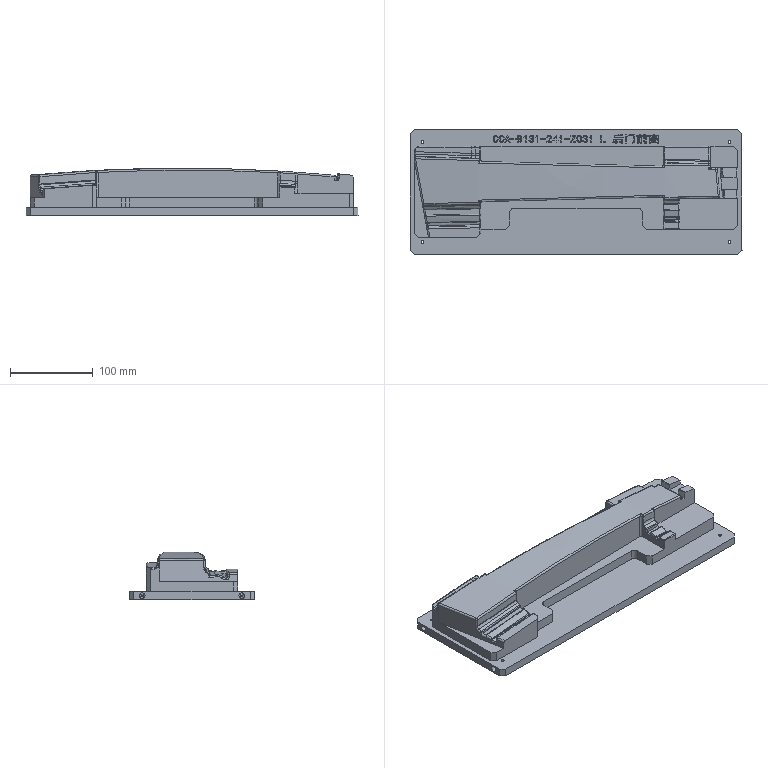NC program | NX | posted with a generic post | part box 400 x 150 x 57.494 mm
Lines 1 to 57 of 7057:
N10 G17 G21 G94 G90
(A1 , TOOL : Z4)
N12 T00 M6
N14 G54
N16 G17 G0 G90 X-185. Y59.998 S1600 M3
N18 G43 Z20.002 H0
N20 G94 G81 G99 Z8.502 F150. R13.002
N22 X-175.885 Y24.394
N24 X-185. Y-60.002
N26 X-152.595 Y-36.192
N28 X-100.084 Y14.254
N30 X0. Y42.744
N32 X96.156 Y-14.266
N34 X131.574 Y21.036
N36 X180. Y42.744
N38 Y-27.256
N40 X185. Y-60.002 Z8.503 R13.003
N42 Y59.998
N44 G80
N46 G0 X185. Y59.998 Z20.003
N48 M5
(A2 , TOOL : Z5)
N50 M6
N52 G54
N54 G17 G0 G90 X-175.885 Y24.394 S1000 M3
N56 G43 Z20.002 H0
N58 G94 G83 G99 Z0.002 F120. Q3. R13.002
N60 X-152.595 Y-36.192
N62 X-100.084 Y14.254
N64 X0. Y42.744
N66 X96.156 Y-14.266
N68 X131.574 Y21.036
N70 X180. Y42.744
N72 Y-27.256
N74 G80
N76 G0 X180. Y-27.256 Z20.002
N78 M5
(A3 , TOOL : Z3.3)
N80 M6
N82 G54
N84 G17 G0 G90 X-185. Y59.998 S1200 M3
N86 G43 Z20.002 H0
N88 G94 G83 G99 Z0.002 F100. Q3. R13.002
N90 Y-60.002
N92 X185. Z0.003 R13.003
N94 Y59.998
N96 G80
N98 G0 X185. Y59.998 Z20.003
N100 M5